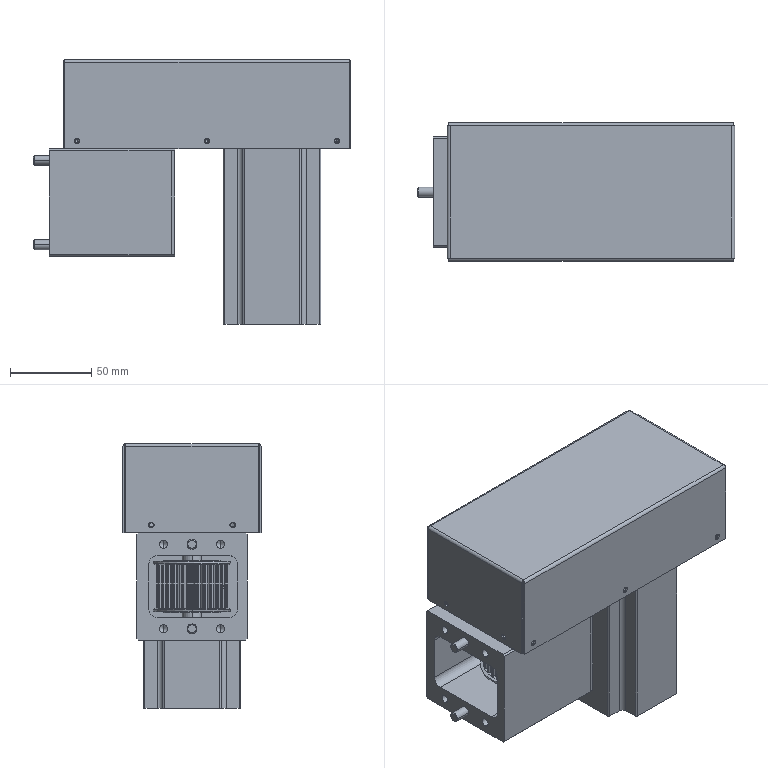Part | SolidWorks | 16 solids | 1493 faces | box 195.5 x 85 x 163 mm | volume 876200 mm3 | cylinder 1102 | plane 184 | cone 147 | torus 60 | commonest cylinder face diameters 1.1 x219 0.5 x216 6.55 x202 59.16 x43 62.7 x42 40.06 x31